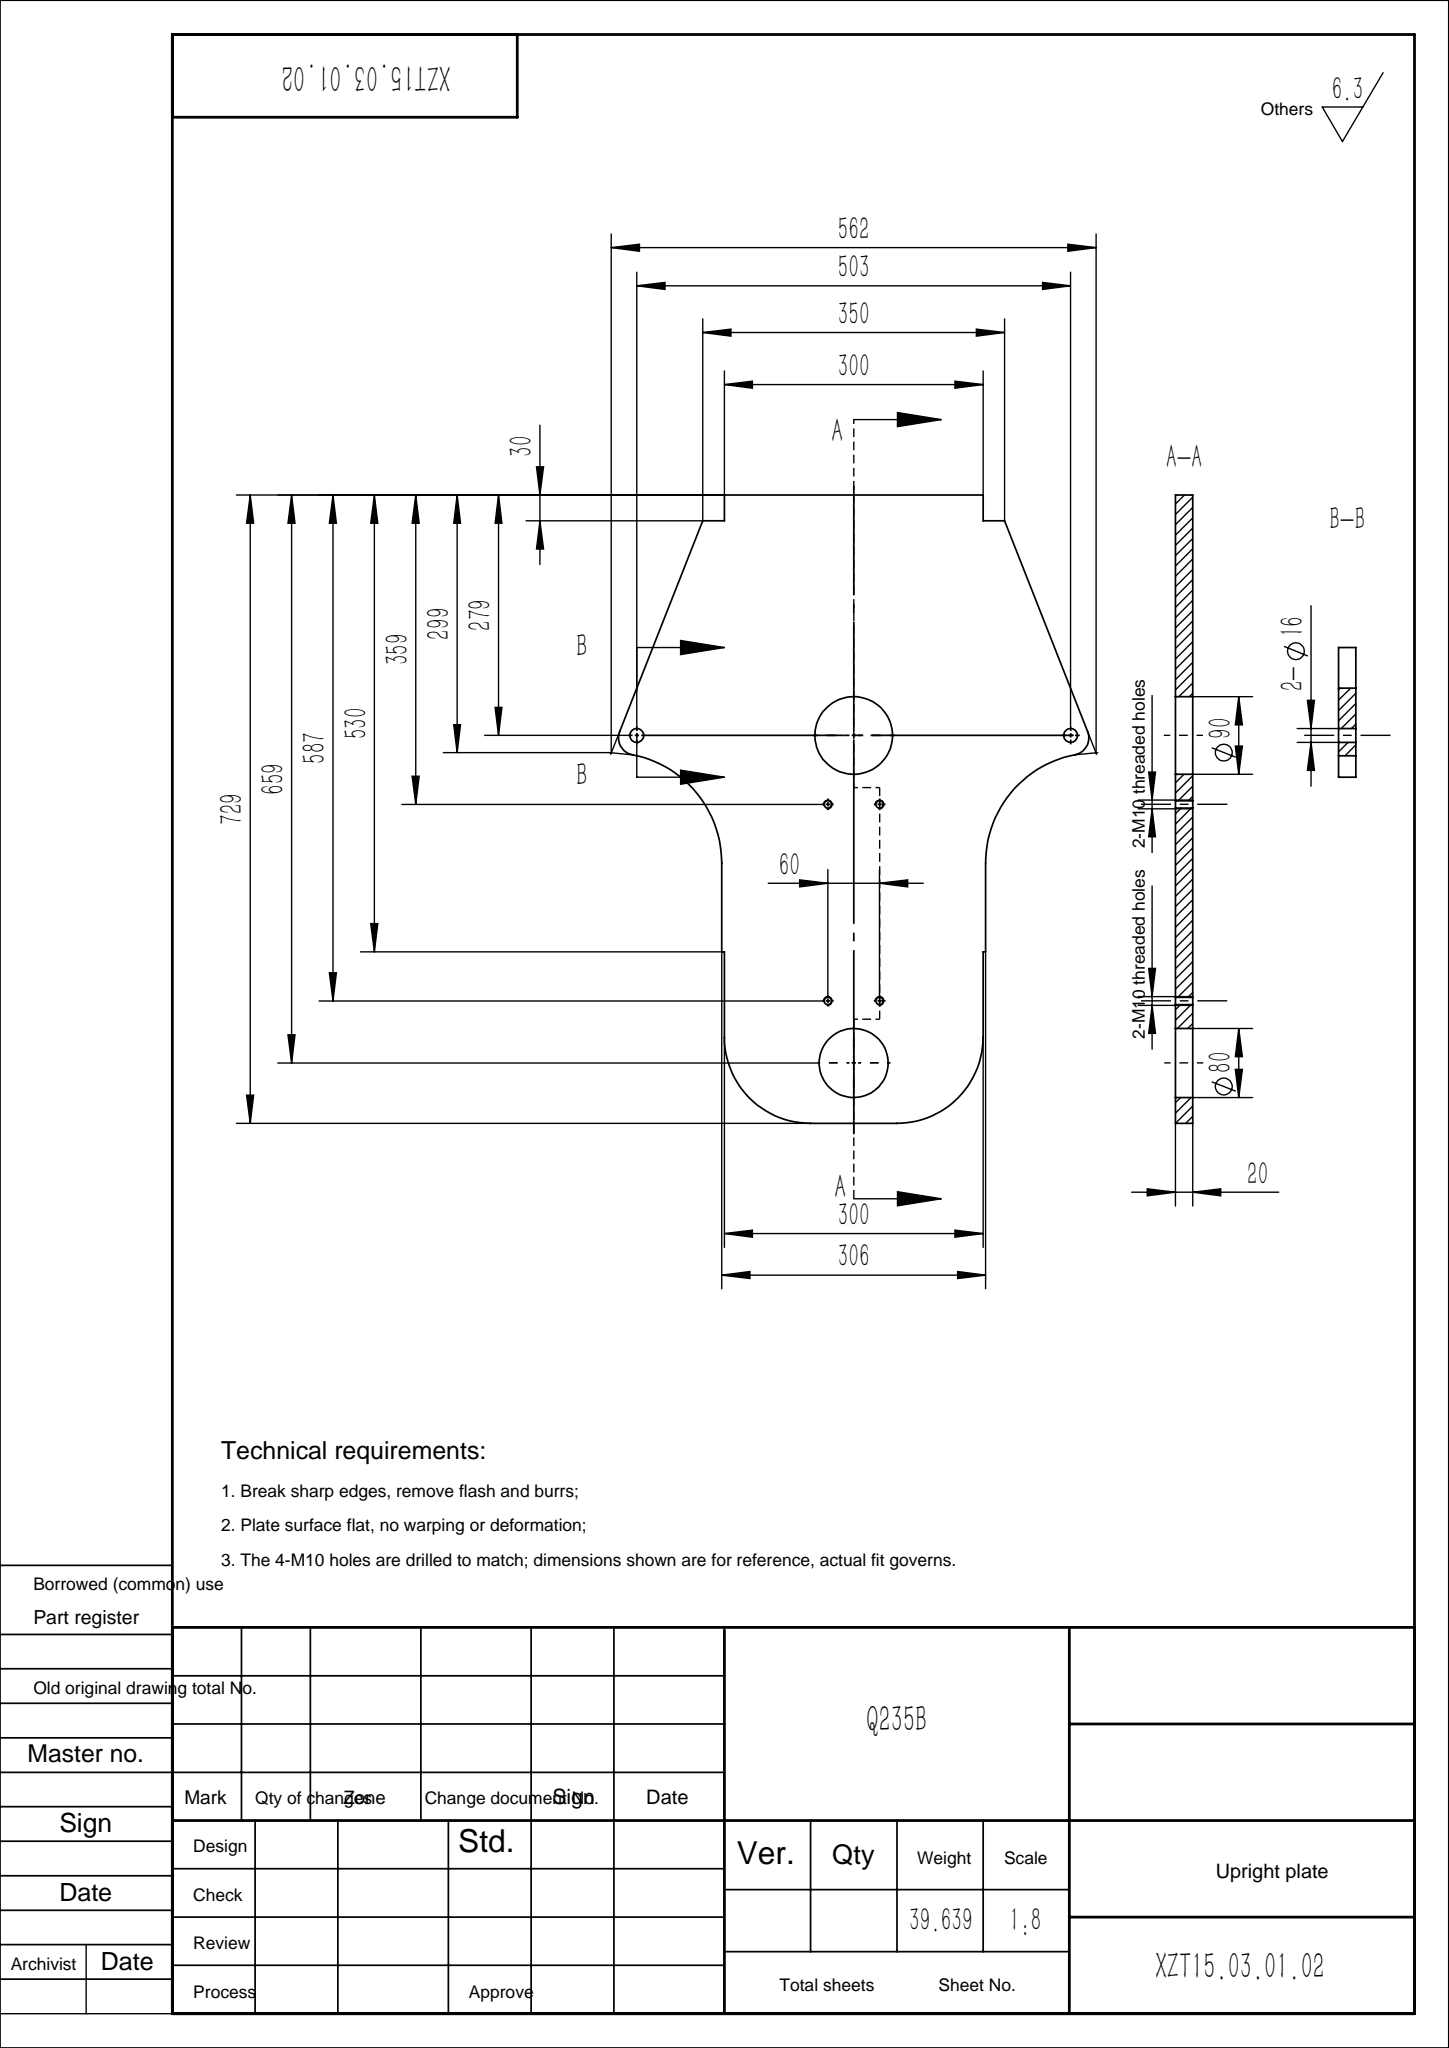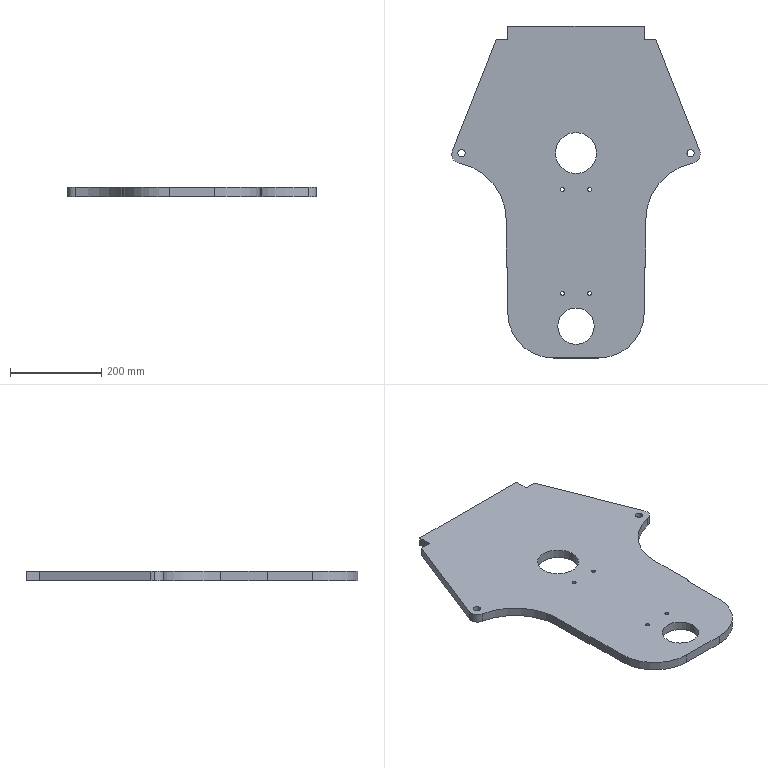Part | SolidWorks | features Fillet 2, Extrusion 1, HoleWzd 1 | 1 solid | 39 faces | box 545.397 x 729 x 20 mm | volume 5049504 mm3 | cylinder 23 | plane 16 | commonest cylinder face diameters 8.5 x8 16 x4 40 x3 80 x2 90 x2 200 x2